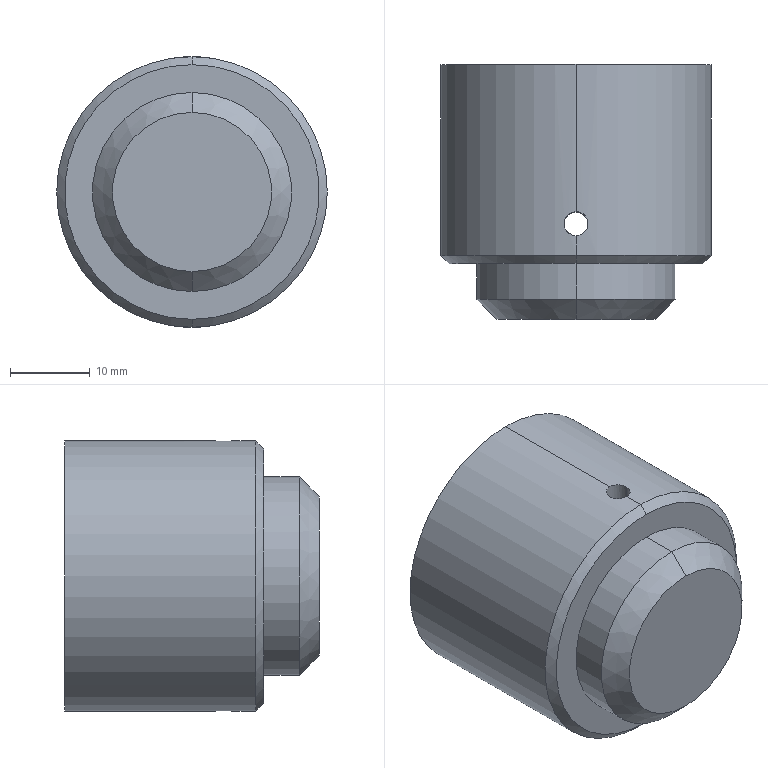Part | SolidWorks | features HoleWzd 1, ICE 1, Revolution 1 | 1 solid | 22 faces | box 34 x 32 x 34 mm | volume 12156 mm3 | cylinder 12 | cone 6 | plane 4 | commonest cylinder face diameters 3 x4 5 x2 25 x2 28 x2 34 x2
STEP:
#1=CARTESIAN_POINT('',(0.,10.5,14.));
#2=VERTEX_POINT('',#1);
#3=CARTESIAN_POINT('',(-1.5,12.,13.919));
#4=VERTEX_POINT('',#3);
#5=CARTESIAN_POINT('',(0.,10.5,14.));
#6=CARTESIAN_POINT('',(-0.09921,10.5,14.));
#7=CARTESIAN_POINT('',(-0.1967,10.51,13.999));
#8=CARTESIAN_POINT('',(-0.3886,10.548,13.995));
#9=CARTESIAN_POINT('',(-0.4839,10.577,13.992));
#10=CARTESIAN_POINT('',(-0.6656,10.652,13.984));
#11=CARTESIAN_POINT('',(-0.7518,10.698,13.98));
#12=CARTESIAN_POINT('',(-0.9148,10.807,13.97));
#13=CARTESIAN_POINT('',(-0.9919,10.871,13.965));
#14=CARTESIAN_POINT('',(-1.199,11.078,13.949));
#15=CARTESIAN_POINT('',(-1.311,11.245,13.939));
#16=CARTESIAN_POINT('',(-1.461,11.607,13.924));
#17=CARTESIAN_POINT('',(-1.5,11.804,13.919));
#18=CARTESIAN_POINT('',(-1.5,12.,13.919));
#19=B_SPLINE_CURVE_WITH_KNOTS('',3,(#5,#6,#7,#8,#9,#10,#11,#12,#13,#14,#15,#16,#17,#18),.UNSPECIFIED.,.F.,.F.,(4,2,2,2,2,2,4),(0.,0.0002934,0.0005868,0.0008802,0.001174,0.00176,0.002347),.UNSPECIFIED.);
#20=EDGE_CURVE('',#2,#4,#19,.T.);
#21=ORIENTED_EDGE('',*,*,#20,.T.);
#22=CARTESIAN_POINT('',(-1.5,12.,16.934));
#23=VERTEX_POINT('',#22);
#24=CARTESIAN_POINT('',(-1.5,12.,-35.));
#25=DIRECTION('',(0.,0.,1.));
#26=VECTOR('',#25,1000.);
#27=LINE('',#24,#26);
#28=EDGE_CURVE('',#4,#23,#27,.T.);
#29=ORIENTED_EDGE('',*,*,#28,.T.);
#30=CARTESIAN_POINT('',(0.,10.5,17.));
#31=VERTEX_POINT('',#30);
#32=CARTESIAN_POINT('',(-1.5,12.,16.934));
#33=CARTESIAN_POINT('',(-1.5,11.802,16.934));
#34=CARTESIAN_POINT('',(-1.461,11.607,16.937));
#35=CARTESIAN_POINT('',(-1.348,11.335,16.947));
#36=CARTESIAN_POINT('',(-1.302,11.249,16.95));
#37=CARTESIAN_POINT('',(-1.193,11.086,16.958));
#38=CARTESIAN_POINT('',(-1.13,11.009,16.963));
#39=CARTESIAN_POINT('',(-0.9228,10.801,16.976));
#40=CARTESIAN_POINT('',(-0.7557,10.69,16.984));
#41=CARTESIAN_POINT('',(-0.3951,10.54,16.996));
#42=CARTESIAN_POINT('',(-0.1982,10.5,17.));
#43=CARTESIAN_POINT('',(0.,10.5,17.));
#44=B_SPLINE_CURVE_WITH_KNOTS('',3,(#32,#33,#34,#35,#36,#37,#38,#39,#40,#41,#42,#43),.UNSPECIFIED.,.F.,.F.,(4,2,2,2,2,4),(0.007039,0.007625,0.007918,0.008211,0.008797,0.009383),.UNSPECIFIED.);
#45=EDGE_CURVE('',#23,#31,#44,.T.);
#46=ORIENTED_EDGE('',*,*,#45,.T.);
#47=CARTESIAN_POINT('',(1.5,12.,16.934));
#48=VERTEX_POINT('',#47);
#49=CARTESIAN_POINT('',(0.,10.5,17.));
#50=CARTESIAN_POINT('',(0.09918,10.5,17.));
#51=CARTESIAN_POINT('',(0.1967,10.51,16.999));
#52=CARTESIAN_POINT('',(0.3885,10.548,16.996));
#53=CARTESIAN_POINT('',(0.4839,10.577,16.993));
#54=CARTESIAN_POINT('',(0.6655,10.652,16.987));
#55=CARTESIAN_POINT('',(0.7517,10.698,16.984));
#56=CARTESIAN_POINT('',(0.9147,10.807,16.976));
#57=CARTESIAN_POINT('',(0.9919,10.871,16.971));
#58=CARTESIAN_POINT('',(1.199,11.078,16.958));
#59=CARTESIAN_POINT('',(1.311,11.246,16.95));
#60=CARTESIAN_POINT('',(1.461,11.607,16.937));
#61=CARTESIAN_POINT('',(1.5,11.804,16.934));
#62=CARTESIAN_POINT('',(1.5,12.,16.934));
#63=B_SPLINE_CURVE_WITH_KNOTS('',3,(#49,#50,#51,#52,#53,#54,#55,#56,#57,#58,#59,#60,#61,#62),.UNSPECIFIED.,.F.,.F.,(4,2,2,2,2,2,4),(0.,0.0002933,0.0005866,0.0008799,0.001173,0.00176,0.002347),.UNSPECIFIED.);
#64=EDGE_CURVE('',#31,#48,#63,.T.);
#65=ORIENTED_EDGE('',*,*,#64,.T.);
#66=CARTESIAN_POINT('',(1.5,12.,13.919));
#67=VERTEX_POINT('',#66);
#68=CARTESIAN_POINT('',(1.5,12.,-35.));
#69=DIRECTION('',(0.,0.,1.));
#70=VECTOR('',#69,1000.);
#71=LINE('',#68,#70);
#72=EDGE_CURVE('',#67,#48,#71,.T.);
#73=ORIENTED_EDGE('',*,*,#72,.F.);
#74=CARTESIAN_POINT('',(1.5,12.,13.919));
#75=CARTESIAN_POINT('',(1.5,11.901,13.919));
#76=CARTESIAN_POINT('',(1.49,11.803,13.92));
#77=CARTESIAN_POINT('',(1.452,11.612,13.924));
#78=CARTESIAN_POINT('',(1.423,11.516,13.928));
#79=CARTESIAN_POINT('',(1.348,11.335,13.935));
#80=CARTESIAN_POINT('',(1.302,11.249,13.939));
#81=CARTESIAN_POINT('',(1.193,11.086,13.949));
#82=CARTESIAN_POINT('',(1.13,11.009,13.954));
#83=CARTESIAN_POINT('',(0.9228,10.801,13.97));
#84=CARTESIAN_POINT('',(0.7558,10.69,13.981));
#85=CARTESIAN_POINT('',(0.3952,10.54,13.996));
#86=CARTESIAN_POINT('',(0.1982,10.5,14.));
#87=CARTESIAN_POINT('',(0.,10.5,14.));
#88=B_SPLINE_CURVE_WITH_KNOTS('',3,(#74,#75,#76,#77,#78,#79,#80,#81,#82,#83,#84,#85,#86,#87),.UNSPECIFIED.,.F.,.F.,(4,2,2,2,2,2,4),(0.00704,0.007333,0.007626,0.007919,0.008213,0.008799,0.009385),.UNSPECIFIED.);
#89=EDGE_CURVE('',#67,#2,#88,.T.);
#90=ORIENTED_EDGE('',*,*,#89,.T.);
#91=EDGE_LOOP('',(#21,#29,#46,#65,#73,#90));
#92=FACE_OUTER_BOUND('',#91,.T.);
#93=CARTESIAN_POINT('',(0.,12.,-35.));
#94=DIRECTION('',(0.,0.,1.));
#95=DIRECTION('',(1.,0.,0.));
#96=AXIS2_PLACEMENT_3D('',#93,#94,#95);
#97=CYLINDRICAL_SURFACE('',#96,1.5);
#98=ADVANCED_FACE('',(#92),#97,.F.);
#99=CARTESIAN_POINT('',(0.,10.5,-17.));
#100=VERTEX_POINT('',#99);
#101=CARTESIAN_POINT('',(-1.5,12.,-16.934));
#102=VERTEX_POINT('',#101);
#103=CARTESIAN_POINT('',(0.,10.5,-17.));
#104=CARTESIAN_POINT('',(-0.09787,10.5,-17.));
#105=CARTESIAN_POINT('',(-0.1973,10.51,-16.999));
#106=CARTESIAN_POINT('',(-0.3896,10.548,-16.996));
#107=CARTESIAN_POINT('',(-0.4831,10.577,-16.993));
#108=CARTESIAN_POINT('',(-0.6648,10.652,-16.987));
#109=CARTESIAN_POINT('',(-0.7525,10.699,-16.984));
#110=CARTESIAN_POINT('',(-0.9149,10.807,-16.976));
#111=CARTESIAN_POINT('',(-0.9907,10.869,-16.971));
#112=CARTESIAN_POINT('',(-1.131,11.009,-16.963));
#113=CARTESIAN_POINT('',(-1.193,11.085,-16.958));
#114=CARTESIAN_POINT('',(-1.301,11.248,-16.95));
#115=CARTESIAN_POINT('',(-1.348,11.335,-16.946));
#116=CARTESIAN_POINT('',(-1.423,11.517,-16.94));
#117=CARTESIAN_POINT('',(-1.452,11.61,-16.938));
#118=CARTESIAN_POINT('',(-1.49,11.803,-16.935));
#119=CARTESIAN_POINT('',(-1.5,11.902,-16.934));
#120=CARTESIAN_POINT('',(-1.5,12.,-16.934));
#121=B_SPLINE_CURVE_WITH_KNOTS('',3,(#103,#104,#105,#106,#107,#108,#109,#110,#111,#112,#113,#114,#115,#116,#117,#118,#119,#120),.UNSPECIFIED.,.F.,.F.,(4,2,2,2,2,2,2,2,4),(0.002347,0.00264,0.002933,0.003226,0.003519,0.003812,0.004106,0.004399,0.004692),.UNSPECIFIED.);
#122=EDGE_CURVE('',#100,#102,#121,.T.);
#123=ORIENTED_EDGE('',*,*,#122,.T.);
#124=CARTESIAN_POINT('',(-1.5,12.,-13.919));
#125=VERTEX_POINT('',#124);
#126=CARTESIAN_POINT('',(-1.5,12.,-35.));
#127=DIRECTION('',(0.,0.,1.));
#128=VECTOR('',#127,1000.);
#129=LINE('',#126,#128);
#130=EDGE_CURVE('',#102,#125,#129,.T.);
#131=ORIENTED_EDGE('',*,*,#130,.T.);
#132=CARTESIAN_POINT('',(0.,10.5,-14.));
#133=VERTEX_POINT('',#132);
#134=CARTESIAN_POINT('',(-1.5,12.,-13.919));
#135=CARTESIAN_POINT('',(-1.5,11.804,-13.919));
#136=CARTESIAN_POINT('',(-1.461,11.607,-13.924));
#137=CARTESIAN_POINT('',(-1.311,11.245,-13.939));
#138=CARTESIAN_POINT('',(-1.199,11.078,-13.949));
#139=CARTESIAN_POINT('',(-0.9918,10.87,-13.965));
#140=CARTESIAN_POINT('',(-0.9147,10.807,-13.97));
#141=CARTESIAN_POINT('',(-0.7517,10.698,-13.98));
#142=CARTESIAN_POINT('',(-0.6656,10.652,-13.984));
#143=CARTESIAN_POINT('',(-0.4839,10.577,-13.992));
#144=CARTESIAN_POINT('',(-0.3886,10.548,-13.995));
#145=CARTESIAN_POINT('',(-0.1967,10.51,-13.999));
#146=CARTESIAN_POINT('',(-0.09918,10.5,-14.));
#147=CARTESIAN_POINT('',(0.,10.5,-14.));
#148=B_SPLINE_CURVE_WITH_KNOTS('',3,(#134,#135,#136,#137,#138,#139,#140,#141,#142,#143,#144,#145,#146,#147),.UNSPECIFIED.,.F.,.F.,(4,2,2,2,2,2,4),(0.004693,0.00528,0.005867,0.00616,0.006453,0.006747,0.00704),.UNSPECIFIED.);
#149=EDGE_CURVE('',#125,#133,#148,.T.);
#150=ORIENTED_EDGE('',*,*,#149,.T.);
#151=CARTESIAN_POINT('',(1.5,12.,-13.919));
#152=VERTEX_POINT('',#151);
#153=CARTESIAN_POINT('',(0.,10.5,-14.));
#154=CARTESIAN_POINT('',(0.09909,10.5,-14.));
#155=CARTESIAN_POINT('',(0.1966,10.51,-13.999));
#156=CARTESIAN_POINT('',(0.3883,10.548,-13.995));
#157=CARTESIAN_POINT('',(0.4835,10.577,-13.992));
#158=CARTESIAN_POINT('',(0.6651,10.652,-13.984));
#159=CARTESIAN_POINT('',(0.7512,10.698,-13.98));
#160=CARTESIAN_POINT('',(0.9141,10.807,-13.97));
#161=CARTESIAN_POINT('',(0.9912,10.87,-13.965));
#162=CARTESIAN_POINT('',(1.199,11.077,-13.949));
#163=CARTESIAN_POINT('',(1.31,11.244,-13.939));
#164=CARTESIAN_POINT('',(1.46,11.605,-13.924));
#165=CARTESIAN_POINT('',(1.5,11.802,-13.919));
#166=CARTESIAN_POINT('',(1.5,12.,-13.919));
#167=B_SPLINE_CURVE_WITH_KNOTS('',3,(#153,#154,#155,#156,#157,#158,#159,#160,#161,#162,#163,#164,#165,#166),.UNSPECIFIED.,.F.,.F.,(4,2,2,2,2,2,4),(0.00704,0.007333,0.007626,0.007919,0.008213,0.008799,0.009385),.UNSPECIFIED.);
#168=EDGE_CURVE('',#133,#152,#167,.T.);
#169=ORIENTED_EDGE('',*,*,#168,.T.);
#170=CARTESIAN_POINT('',(1.5,12.,-16.934));
#171=VERTEX_POINT('',#170);
#172=CARTESIAN_POINT('',(1.5,12.,-35.));
#173=DIRECTION('',(0.,0.,1.));
#174=VECTOR('',#173,1000.);
#175=LINE('',#172,#174);
#176=EDGE_CURVE('',#171,#152,#175,.T.);
#177=ORIENTED_EDGE('',*,*,#176,.F.);
#178=CARTESIAN_POINT('',(1.5,12.,-16.934));
#179=CARTESIAN_POINT('',(1.5,11.901,-16.934));
#180=CARTESIAN_POINT('',(1.49,11.803,-16.935));
#181=CARTESIAN_POINT('',(1.452,11.611,-16.938));
#182=CARTESIAN_POINT('',(1.423,11.516,-16.94));
#183=CARTESIAN_POINT('',(1.348,11.334,-16.947));
#184=CARTESIAN_POINT('',(1.302,11.248,-16.95));
#185=CARTESIAN_POINT('',(1.193,11.085,-16.958));
#186=CARTESIAN_POINT('',(1.129,11.008,-16.963));
#187=CARTESIAN_POINT('',(0.9219,10.801,-16.976));
#188=CARTESIAN_POINT('',(0.7545,10.689,-16.984));
#189=CARTESIAN_POINT('',(0.3934,10.539,-16.996));
#190=CARTESIAN_POINT('',(0.1958,10.5,-17.));
#191=CARTESIAN_POINT('',(0.,10.5,-17.));
#192=B_SPLINE_CURVE_WITH_KNOTS('',3,(#178,#179,#180,#181,#182,#183,#184,#185,#186,#187,#188,#189,#190,#191),.UNSPECIFIED.,.F.,.F.,(4,2,2,2,2,2,4),(0.,0.0002933,0.0005866,0.0008799,0.001173,0.00176,0.002347),.UNSPECIFIED.);
#193=EDGE_CURVE('',#171,#100,#192,.T.);
#194=ORIENTED_EDGE('',*,*,#193,.T.);
#195=EDGE_LOOP('',(#123,#131,#150,#169,#177,#194));
#196=FACE_OUTER_BOUND('',#195,.T.);
#197=CARTESIAN_POINT('',(0.,12.,-35.));
#198=DIRECTION('',(0.,0.,1.));
#199=DIRECTION('',(1.,0.,0.));
#200=AXIS2_PLACEMENT_3D('',#197,#198,#199);
#201=CYLINDRICAL_SURFACE('',#200,1.5);
#202=ADVANCED_FACE('',(#196),#201,.F.);
#203=CARTESIAN_POINT('',(0.,5.,-2.5));
#204=VERTEX_POINT('',#203);
#205=CARTESIAN_POINT('',(0.,5.,2.5));
#206=VERTEX_POINT('',#205);
#207=CARTESIAN_POINT('',(0.,5.,0.));
#208=DIRECTION('',(0.,1.,0.));
#209=DIRECTION('',(0.,0.,1.));
#210=AXIS2_PLACEMENT_3D('',#207,#208,#209);
#211=CIRCLE('',#210,2.5);
#212=EDGE_CURVE('',#204,#206,#211,.T.);
#213=ORIENTED_EDGE('',*,*,#212,.F.);
#214=CARTESIAN_POINT('',(0.,10.,-2.5));
#215=VERTEX_POINT('',#214);
#216=CARTESIAN_POINT('',(0.,10.,-2.5));
#217=DIRECTION('',(0.,1.,0.));
#218=VECTOR('',#217,1000.);
#219=LINE('',#216,#218);
#220=EDGE_CURVE('',#204,#215,#219,.T.);
#221=ORIENTED_EDGE('',*,*,#220,.T.);
#222=CARTESIAN_POINT('',(0.,10.,2.5));
#223=VERTEX_POINT('',#222);
#224=CARTESIAN_POINT('',(0.,10.,0.));
#225=DIRECTION('',(0.,1.,0.));
#226=DIRECTION('',(0.,0.,1.));
#227=AXIS2_PLACEMENT_3D('',#224,#225,#226);
#228=CIRCLE('',#227,2.5);
#229=EDGE_CURVE('',#215,#223,#228,.T.);
#230=ORIENTED_EDGE('',*,*,#229,.T.);
#231=CARTESIAN_POINT('',(0.,10.,2.5));
#232=DIRECTION('',(0.,1.,0.));
#233=VECTOR('',#232,1000.);
#234=LINE('',#231,#233);
#235=EDGE_CURVE('',#206,#223,#234,.T.);
#236=ORIENTED_EDGE('',*,*,#235,.F.);
#237=EDGE_LOOP('',(#213,#221,#230,#236));
#238=FACE_OUTER_BOUND('',#237,.T.);
#239=CARTESIAN_POINT('',(0.,10.,0.));
#240=DIRECTION('',(0.,1.,0.));
#241=DIRECTION('',(0.,0.,1.));
#242=AXIS2_PLACEMENT_3D('',#239,#240,#241);
#243=CYLINDRICAL_SURFACE('',#242,2.5);
#244=ADVANCED_FACE('',(#238),#243,.F.);
#245=CARTESIAN_POINT('',(0.,3.498,0.));
#246=VERTEX_POINT('',#245);
#247=CARTESIAN_POINT('',(0.,5.,2.5));
#248=DIRECTION('',(0.,0.515,0.8572));
#249=VECTOR('',#248,1000.);
#250=LINE('',#247,#249);
#251=EDGE_CURVE('',#246,#206,#250,.T.);
#252=ORIENTED_EDGE('',*,*,#251,.F.);
#253=CARTESIAN_POINT('',(0.,5.,-2.5));
#254=DIRECTION('',(0.,0.515,-0.8572));
#255=VECTOR('',#254,1000.);
#256=LINE('',#253,#255);
#257=EDGE_CURVE('',#246,#204,#256,.T.);
#258=ORIENTED_EDGE('',*,*,#257,.T.);
#259=ORIENTED_EDGE('',*,*,#212,.T.);
#260=EDGE_LOOP('',(#252,#258,#259));
#261=FACE_OUTER_BOUND('',#260,.T.);
#262=CARTESIAN_POINT('',(0.,5.,0.));
#263=DIRECTION('',(0.,1.,0.));
#264=DIRECTION('',(0.,0.,1.));
#265=AXIS2_PLACEMENT_3D('',#262,#263,#264);
#266=CONICAL_SURFACE('',#265,2.5,1.03);
#267=ADVANCED_FACE('',(#261),#266,.F.);
#268=CARTESIAN_POINT('',(0.,10.,-14.));
#269=VERTEX_POINT('',#268);
#270=CARTESIAN_POINT('',(0.,10.,14.));
#271=VERTEX_POINT('',#270);
#272=CARTESIAN_POINT('',(0.,10.,0.));
#273=DIRECTION('',(0.,1.,0.));
#274=DIRECTION('',(0.,0.,1.));
#275=AXIS2_PLACEMENT_3D('',#272,#273,#274);
#276=CIRCLE('',#275,14.);
#277=EDGE_CURVE('',#269,#271,#276,.T.);
#278=ORIENTED_EDGE('',*,*,#277,.F.);
#279=CARTESIAN_POINT('',(0.,19.381,-14.));
#280=DIRECTION('',(0.,1.,0.));
#281=VECTOR('',#280,1000.);
#282=LINE('',#279,#281);
#283=EDGE_CURVE('',#269,#133,#282,.T.);
#284=ORIENTED_EDGE('',*,*,#283,.T.);
#285=ORIENTED_EDGE('',*,*,#149,.F.);
#286=CARTESIAN_POINT('',(0.,13.5,-14.));
#287=VERTEX_POINT('',#286);
#288=CARTESIAN_POINT('',(0.,13.5,-14.));
#289=CARTESIAN_POINT('',(-0.09789,13.5,-14.));
#290=CARTESIAN_POINT('',(-0.1973,13.49,-13.999));
#291=CARTESIAN_POINT('',(-0.3897,13.452,-13.995));
#292=CARTESIAN_POINT('',(-0.4832,13.423,-13.992));
#293=CARTESIAN_POINT('',(-0.6649,13.348,-13.984));
#294=CARTESIAN_POINT('',(-0.7526,13.301,-13.98));
#295=CARTESIAN_POINT('',(-0.915,13.193,-13.97));
#296=CARTESIAN_POINT('',(-0.9907,13.131,-13.965));
#297=CARTESIAN_POINT('',(-1.131,12.991,-13.954));
#298=CARTESIAN_POINT('',(-1.193,12.915,-13.949));
#299=CARTESIAN_POINT('',(-1.301,12.753,-13.94));
#300=CARTESIAN_POINT('',(-1.348,12.665,-13.935));
#301=CARTESIAN_POINT('',(-1.423,12.483,-13.927));
#302=CARTESIAN_POINT('',(-1.452,12.39,-13.925));
#303=CARTESIAN_POINT('',(-1.49,12.197,-13.92));
#304=CARTESIAN_POINT('',(-1.5,12.098,-13.919));
#305=CARTESIAN_POINT('',(-1.5,12.,-13.919));
#306=B_SPLINE_CURVE_WITH_KNOTS('',3,(#288,#289,#290,#291,#292,#293,#294,#295,#296,#297,#298,#299,#300,#301,#302,#303,#304,#305),.UNSPECIFIED.,.F.,.F.,(4,2,2,2,2,2,2,2,4),(0.002347,0.00264,0.002934,0.003227,0.00352,0.003813,0.004107,0.0044,0.004693),.UNSPECIFIED.);
#307=EDGE_CURVE('',#287,#125,#306,.T.);
#308=ORIENTED_EDGE('',*,*,#307,.F.);
#309=CARTESIAN_POINT('',(0.,32.,-14.));
#310=VERTEX_POINT('',#309);
#311=CARTESIAN_POINT('',(0.,19.381,-14.));
#312=DIRECTION('',(0.,1.,0.));
#313=VECTOR('',#312,1000.);
#314=LINE('',#311,#313);
#315=EDGE_CURVE('',#287,#310,#314,.T.);
#316=ORIENTED_EDGE('',*,*,#315,.T.);
#317=CARTESIAN_POINT('',(0.,32.,14.));
#318=VERTEX_POINT('',#317);
#319=CARTESIAN_POINT('',(0.,32.,0.));
#320=DIRECTION('',(0.,1.,0.));
#321=DIRECTION('',(0.,0.,1.));
#322=AXIS2_PLACEMENT_3D('',#319,#320,#321);
#323=CIRCLE('',#322,14.);
#324=EDGE_CURVE('',#310,#318,#323,.T.);
#325=ORIENTED_EDGE('',*,*,#324,.T.);
#326=CARTESIAN_POINT('',(0.,13.5,14.));
#327=VERTEX_POINT('',#326);
#328=CARTESIAN_POINT('',(0.,19.381,14.));
#329=DIRECTION('',(0.,1.,0.));
#330=VECTOR('',#329,1000.);
#331=LINE('',#328,#330);
#332=EDGE_CURVE('',#327,#318,#331,.T.);
#333=ORIENTED_EDGE('',*,*,#332,.F.);
#334=CARTESIAN_POINT('',(-1.5,12.,13.919));
#335=CARTESIAN_POINT('',(-1.5,12.098,13.919));
#336=CARTESIAN_POINT('',(-1.49,12.197,13.92));
#337=CARTESIAN_POINT('',(-1.452,12.39,13.925));
#338=CARTESIAN_POINT('',(-1.423,12.483,13.928));
#339=CARTESIAN_POINT('',(-1.348,12.665,13.935));
#340=CARTESIAN_POINT('',(-1.301,12.753,13.94));
#341=CARTESIAN_POINT('',(-1.193,12.915,13.949));
#342=CARTESIAN_POINT('',(-1.131,12.991,13.954));
#343=CARTESIAN_POINT('',(-0.9906,13.131,13.965));
#344=CARTESIAN_POINT('',(-0.9149,13.193,13.97));
#345=CARTESIAN_POINT('',(-0.7525,13.301,13.98));
#346=CARTESIAN_POINT('',(-0.6648,13.348,13.985));
#347=CARTESIAN_POINT('',(-0.4832,13.423,13.992));
#348=CARTESIAN_POINT('',(-0.3897,13.452,13.995));
#349=CARTESIAN_POINT('',(-0.1974,13.49,13.999));
#350=CARTESIAN_POINT('',(-0.09791,13.5,14.));
#351=CARTESIAN_POINT('',(0.,13.5,14.));
#352=B_SPLINE_CURVE_WITH_KNOTS('',3,(#334,#335,#336,#337,#338,#339,#340,#341,#342,#343,#344,#345,#346,#347,#348,#349,#350,#351),.UNSPECIFIED.,.F.,.F.,(4,2,2,2,2,2,2,2,4),(0.002347,0.00264,0.002934,0.003227,0.00352,0.003813,0.004107,0.0044,0.004693),.UNSPECIFIED.);
#353=EDGE_CURVE('',#4,#327,#352,.T.);
#354=ORIENTED_EDGE('',*,*,#353,.F.);
#355=ORIENTED_EDGE('',*,*,#20,.F.);
#356=CARTESIAN_POINT('',(0.,19.381,14.));
#357=DIRECTION('',(0.,1.,0.));
#358=VECTOR('',#357,1000.);
#359=LINE('',#356,#358);
#360=EDGE_CURVE('',#271,#2,#359,.T.);
#361=ORIENTED_EDGE('',*,*,#360,.F.);
#362=EDGE_LOOP('',(#278,#284,#285,#308,#316,#325,#333,#354,#355,#361));
#363=FACE_OUTER_BOUND('',#362,.T.);
#364=CARTESIAN_POINT('',(0.,19.381,0.));
#365=DIRECTION('',(0.,1.,0.));
#366=DIRECTION('',(0.,0.,1.));
#367=AXIS2_PLACEMENT_3D('',#364,#365,#366);
#368=CYLINDRICAL_SURFACE('',#367,14.);
#369=ADVANCED_FACE('',(#363),#368,.F.);
#370=CARTESIAN_POINT('',(0.,8.,17.));
#371=VERTEX_POINT('',#370);
#372=CARTESIAN_POINT('',(0.,8.,-17.));
#373=VERTEX_POINT('',#372);
#374=CARTESIAN_POINT('',(0.,8.,0.));
#375=DIRECTION('',(0.,1.,0.));
#376=DIRECTION('',(0.,0.,1.));
#377=AXIS2_PLACEMENT_3D('',#374,#375,#376);
#378=CIRCLE('',#377,17.);
#379=EDGE_CURVE('',#371,#373,#378,.T.);
#380=ORIENTED_EDGE('',*,*,#379,.T.);
#381=CARTESIAN_POINT('',(0.,19.381,-17.));
#382=DIRECTION('',(0.,1.,0.));
#383=VECTOR('',#382,1000.);
#384=LINE('',#381,#383);
#385=EDGE_CURVE('',#373,#100,#384,.T.);
#386=ORIENTED_EDGE('',*,*,#385,.T.);
#387=ORIENTED_EDGE('',*,*,#193,.F.);
#388=CARTESIAN_POINT('',(0.,13.5,-17.));
#389=VERTEX_POINT('',#388);
#390=CARTESIAN_POINT('',(0.,13.5,-17.));
#391=CARTESIAN_POINT('',(0.198,13.5,-17.));
#392=CARTESIAN_POINT('',(0.3926,13.461,-16.996));
#393=CARTESIAN_POINT('',(0.665,13.348,-16.987));
#394=CARTESIAN_POINT('',(0.7511,13.302,-16.984));
#395=CARTESIAN_POINT('',(0.914,13.193,-16.976));
#396=CARTESIAN_POINT('',(0.9912,13.13,-16.971));
#397=CARTESIAN_POINT('',(1.199,12.923,-16.958));
#398=CARTESIAN_POINT('',(1.31,12.756,-16.95));
#399=CARTESIAN_POINT('',(1.46,12.395,-16.937));
#400=CARTESIAN_POINT('',(1.5,12.198,-16.934));
#401=CARTESIAN_POINT('',(1.5,12.,-16.934));
#402=B_SPLINE_CURVE_WITH_KNOTS('',3,(#390,#391,#392,#393,#394,#395,#396,#397,#398,#399,#400,#401),.UNSPECIFIED.,.F.,.F.,(4,2,2,2,2,4),(0.007039,0.007625,0.007918,0.008211,0.008797,0.009383),.UNSPECIFIED.);
#403=EDGE_CURVE('',#389,#171,#402,.T.);
#404=ORIENTED_EDGE('',*,*,#403,.F.);
#405=CARTESIAN_POINT('',(0.,32.,-17.));
#406=VERTEX_POINT('',#405);
#407=CARTESIAN_POINT('',(0.,19.381,-17.));
#408=DIRECTION('',(0.,1.,0.));
#409=VECTOR('',#408,1000.);
#410=LINE('',#407,#409);
#411=EDGE_CURVE('',#389,#406,#410,.T.);
#412=ORIENTED_EDGE('',*,*,#411,.T.);
#413=CARTESIAN_POINT('',(0.,32.,17.));
#414=VERTEX_POINT('',#413);
#415=CARTESIAN_POINT('',(0.,32.,0.));
#416=DIRECTION('',(0.,1.,0.));
#417=DIRECTION('',(0.,0.,1.));
#418=AXIS2_PLACEMENT_3D('',#415,#416,#417);
#419=CIRCLE('',#418,17.);
#420=EDGE_CURVE('',#414,#406,#419,.T.);
#421=ORIENTED_EDGE('',*,*,#420,.F.);
#422=CARTESIAN_POINT('',(0.,13.5,17.));
#423=VERTEX_POINT('',#422);
#424=CARTESIAN_POINT('',(0.,19.381,17.));
#425=DIRECTION('',(0.,1.,0.));
#426=VECTOR('',#425,1000.);
#427=LINE('',#424,#426);
#428=EDGE_CURVE('',#423,#414,#427,.T.);
#429=ORIENTED_EDGE('',*,*,#428,.F.);
#430=CARTESIAN_POINT('',(1.5,12.,16.934));
#431=CARTESIAN_POINT('',(1.5,12.098,16.934));
#432=CARTESIAN_POINT('',(1.49,12.197,16.935));
#433=CARTESIAN_POINT('',(1.452,12.39,16.938));
#434=CARTESIAN_POINT('',(1.423,12.483,16.94));
#435=CARTESIAN_POINT('',(1.348,12.665,16.946));
#436=CARTESIAN_POINT('',(1.301,12.752,16.95));
#437=CARTESIAN_POINT('',(1.193,12.915,16.958));
#438=CARTESIAN_POINT('',(1.131,12.991,16.963));
#439=CARTESIAN_POINT('',(0.9906,13.131,16.971));
#440=CARTESIAN_POINT('',(0.9149,13.193,16.976));
#441=CARTESIAN_POINT('',(0.7525,13.301,16.984));
#442=CARTESIAN_POINT('',(0.6648,13.348,16.987));
#443=CARTESIAN_POINT('',(0.4831,13.423,16.993));
#444=CARTESIAN_POINT('',(0.3896,13.452,16.996));
#445=CARTESIAN_POINT('',(0.1973,13.49,16.999));
#446=CARTESIAN_POINT('',(0.0979,13.5,17.));
#447=CARTESIAN_POINT('',(0.,13.5,17.));
#448=B_SPLINE_CURVE_WITH_KNOTS('',3,(#430,#431,#432,#433,#434,#435,#436,#437,#438,#439,#440,#441,#442,#443,#444,#445,#446,#447),.UNSPECIFIED.,.F.,.F.,(4,2,2,2,2,2,2,2,4),(0.002347,0.00264,0.002933,0.003226,0.003519,0.003812,0.004106,0.004399,0.004692),.UNSPECIFIED.);
#449=EDGE_CURVE('',#48,#423,#448,.T.);
#450=ORIENTED_EDGE('',*,*,#449,.F.);
#451=ORIENTED_EDGE('',*,*,#64,.F.);
#452=CARTESIAN_POINT('',(0.,19.381,17.));
#453=DIRECTION('',(0.,1.,0.));
#454=VECTOR('',#453,1000.);
#455=LINE('',#452,#454);
#456=EDGE_CURVE('',#371,#31,#455,.T.);
#457=ORIENTED_EDGE('',*,*,#456,.F.);
#458=EDGE_LOOP('',(#380,#386,#387,#404,#412,#421,#429,#450,#451,#457));
#459=FACE_OUTER_BOUND('',#458,.T.);
#460=CARTESIAN_POINT('',(0.,19.381,0.));
#461=DIRECTION('',(0.,1.,0.));
#462=DIRECTION('',(0.,0.,1.));
#463=AXIS2_PLACEMENT_3D('',#460,#461,#462);
#464=CYLINDRICAL_SURFACE('',#463,17.);
#465=ADVANCED_FACE('',(#459),#464,.T.);
#466=CARTESIAN_POINT('',(0.,7.,16.));
#467=VERTEX_POINT('',#466);
#468=CARTESIAN_POINT('',(0.,7.,-16.));
#469=VERTEX_POINT('',#468);
#470=CARTESIAN_POINT('',(0.,7.,0.));
#471=DIRECTION('',(0.,1.,0.));
#472=DIRECTION('',(0.,0.,1.));
#473=AXIS2_PLACEMENT_3D('',#470,#471,#472);
#474=CIRCLE('',#473,16.);
#475=EDGE_CURVE('',#467,#469,#474,.T.);
#476=ORIENTED_EDGE('',*,*,#475,.T.);
#477=CARTESIAN_POINT('',(0.,8.,-17.));
#478=DIRECTION('',(0.,0.7071,-0.7071));
#479=VECTOR('',#478,1000.);
#480=LINE('',#477,#479);
#481=EDGE_CURVE('',#469,#373,#480,.T.);
#482=ORIENTED_EDGE('',*,*,#481,.T.);
#483=ORIENTED_EDGE('',*,*,#379,.F.);
#484=CARTESIAN_POINT('',(0.,8.,17.));
#485=DIRECTION('',(0.,0.7071,0.7071));
#486=VECTOR('',#485,1000.);
#487=LINE('',#484,#486);
#488=EDGE_CURVE('',#467,#371,#487,.T.);
#489=ORIENTED_EDGE('',*,*,#488,.F.);
#490=EDGE_LOOP('',(#476,#482,#483,#489));
#491=FACE_OUTER_BOUND('',#490,.T.);
#492=CARTESIAN_POINT('',(0.,8.,0.));
#493=DIRECTION('',(0.,1.,0.));
#494=DIRECTION('',(0.,0.,1.));
#495=AXIS2_PLACEMENT_3D('',#492,#493,#494);
#496=CONICAL_SURFACE('',#495,17.,0.7854);
#497=ADVANCED_FACE('',(#491),#496,.T.);
#498=CARTESIAN_POINT('',(0.,2.5,12.5));
#499=VERTEX_POINT('',#498);
#500=CARTESIAN_POINT('',(0.,2.5,-12.5));
#501=VERTEX_POINT('',#500);
#502=CARTESIAN_POINT('',(0.,2.5,0.));
#503=DIRECTION('',(0.,1.,0.));
#504=DIRECTION('',(0.,0.,1.));
#505=AXIS2_PLACEMENT_3D('',#502,#503,#504);
#506=CIRCLE('',#505,12.5);
#507=EDGE_CURVE('',#499,#501,#506,.T.);
#508=ORIENTED_EDGE('',*,*,#507,.T.);
#509=CARTESIAN_POINT('',(0.,7.,-12.5));
#510=VERTEX_POINT('',#509);
#511=CARTESIAN_POINT('',(0.,19.381,-12.5));
#512=DIRECTION('',(0.,1.,0.));
#513=VECTOR('',#512,1000.);
#514=LINE('',#511,#513);
#515=EDGE_CURVE('',#501,#510,#514,.T.);
#516=ORIENTED_EDGE('',*,*,#515,.T.);
#517=CARTESIAN_POINT('',(0.,7.,12.5));
#518=VERTEX_POINT('',#517);
#519=CARTESIAN_POINT('',(0.,7.,0.));
#520=DIRECTION('',(0.,1.,0.));
#521=DIRECTION('',(0.,0.,1.));
#522=AXIS2_PLACEMENT_3D('',#519,#520,#521);
#523=CIRCLE('',#522,12.5);
#524=EDGE_CURVE('',#518,#510,#523,.T.);
#525=ORIENTED_EDGE('',*,*,#524,.F.);
#526=CARTESIAN_POINT('',(0.,19.381,12.5));
#527=DIRECTION('',(0.,1.,0.));
#528=VECTOR('',#527,1000.);
#529=LINE('',#526,#528);
#530=EDGE_CURVE('',#499,#518,#529,.T.);
#531=ORIENTED_EDGE('',*,*,#530,.F.);
#532=EDGE_LOOP('',(#508,#516,#525,#531));
#533=FACE_OUTER_BOUND('',#532,.T.);
#534=CARTESIAN_POINT('',(0.,19.381,0.));
#535=DIRECTION('',(0.,1.,0.));
#536=DIRECTION('',(0.,0.,1.));
#537=AXIS2_PLACEMENT_3D('',#534,#535,#536);
#538=CYLINDRICAL_SURFACE('',#537,12.5);
#539=ADVANCED_FACE('',(#533),#538,.T.);
#540=CARTESIAN_POINT('',(0.,0.,10.));
#541=VERTEX_POINT('',#540);
#542=CARTESIAN_POINT('',(0.,0.,-10.));
#543=VERTEX_POINT('',#542);
#544=CARTESIAN_POINT('',(0.,0.,0.));
#545=DIRECTION('',(0.,1.,0.));
#546=DIRECTION('',(0.,0.,1.));
#547=AXIS2_PLACEMENT_3D('',#544,#545,#546);
#548=CIRCLE('',#547,10.);
#549=EDGE_CURVE('',#541,#543,#548,.T.);
#550=ORIENTED_EDGE('',*,*,#549,.T.);
#551=CARTESIAN_POINT('',(0.,2.5,-12.5));
#552=DIRECTION('',(0.,0.7071,-0.7071));
#553=VECTOR('',#552,1000.);
#554=LINE('',#551,#553);
#555=EDGE_CURVE('',#543,#501,#554,.T.);
#556=ORIENTED_EDGE('',*,*,#555,.T.);
#557=ORIENTED_EDGE('',*,*,#507,.F.);
#558=CARTESIAN_POINT('',(0.,2.5,12.5));
#559=DIRECTION('',(0.,0.7071,0.7071));
#560=VECTOR('',#559,1000.);
#561=LINE('',#558,#560);
#562=EDGE_CURVE('',#541,#499,#561,.T.);
#563=ORIENTED_EDGE('',*,*,#562,.F.);
#564=EDGE_LOOP('',(#550,#556,#557,#563));
#565=FACE_OUTER_BOUND('',#564,.T.);
#566=CARTESIAN_POINT('',(0.,2.5,0.));
#567=DIRECTION('',(0.,1.,0.));
#568=DIRECTION('',(0.,0.,1.));
#569=AXIS2_PLACEMENT_3D('',#566,#567,#568);
#570=CONICAL_SURFACE('',#569,12.5,0.7854);
#571=ADVANCED_FACE('',(#565),#570,.T.);
#572=ORIENTED_EDGE('',*,*,#549,.F.);
#573=CARTESIAN_POINT('',(0.,0.,0.));
#574=DIRECTION('',(0.,1.,0.));
#575=DIRECTION('',(0.,0.,1.));
#576=AXIS2_PLACEMENT_3D('',#573,#574,#575);
#577=CIRCLE('',#576,10.);
#578=EDGE_CURVE('',#543,#541,#577,.T.);
#579=ORIENTED_EDGE('',*,*,#578,.F.);
#580=EDGE_LOOP('',(#572,#579));
#581=FACE_OUTER_BOUND('',#580,.T.);
#582=CARTESIAN_POINT('',(0.,0.,0.));
#583=DIRECTION('',(0.,-1.,0.));
#584=DIRECTION('',(0.,0.,-1.));
#585=AXIS2_PLACEMENT_3D('',#582,#583,#584);
#586=PLANE('',#585);
#587=ADVANCED_FACE('',(#581),#586,.T.);
#588=ORIENTED_EDGE('',*,*,#555,.F.);
#589=ORIENTED_EDGE('',*,*,#578,.T.);
#590=ORIENTED_EDGE('',*,*,#562,.T.);
#591=CARTESIAN_POINT('',(0.,2.5,0.));
#592=DIRECTION('',(0.,1.,0.));
#593=DIRECTION('',(0.,0.,1.));
#594=AXIS2_PLACEMENT_3D('',#591,#592,#593);
#595=CIRCLE('',#594,12.5);
#596=EDGE_CURVE('',#501,#499,#595,.T.);
#597=ORIENTED_EDGE('',*,*,#596,.F.);
#598=EDGE_LOOP('',(#588,#589,#590,#597));
#599=FACE_OUTER_BOUND('',#598,.T.);
#600=CARTESIAN_POINT('',(0.,2.5,0.));
#601=DIRECTION('',(0.,1.,0.));
#602=DIRECTION('',(0.,0.,1.));
#603=AXIS2_PLACEMENT_3D('',#600,#601,#602);
#604=CONICAL_SURFACE('',#603,12.5,0.7854);
#605=ADVANCED_FACE('',(#599),#604,.T.);
#606=ORIENTED_EDGE('',*,*,#515,.F.);
#607=ORIENTED_EDGE('',*,*,#596,.T.);
#608=ORIENTED_EDGE('',*,*,#530,.T.);
#609=CARTESIAN_POINT('',(0.,7.,0.));
#610=DIRECTION('',(0.,1.,0.));
#611=DIRECTION('',(0.,0.,1.));
#612=AXIS2_PLACEMENT_3D('',#609,#610,#611);
#613=CIRCLE('',#612,12.5);
#614=EDGE_CURVE('',#510,#518,#613,.T.);
#615=ORIENTED_EDGE('',*,*,#614,.F.);
#616=EDGE_LOOP('',(#606,#607,#608,#615));
#617=FACE_OUTER_BOUND('',#616,.T.);
#618=CARTESIAN_POINT('',(0.,19.381,0.));
#619=DIRECTION('',(0.,1.,0.));
#620=DIRECTION('',(0.,0.,1.));
#621=AXIS2_PLACEMENT_3D('',#618,#619,#620);
#622=CYLINDRICAL_SURFACE('',#621,12.5);
#623=ADVANCED_FACE('',(#617),#622,.T.);
#624=ORIENTED_EDGE('',*,*,#524,.T.);
#625=ORIENTED_EDGE('',*,*,#614,.T.);
#626=EDGE_LOOP('',(#624,#625));
#627=FACE_BOUND('',#626,.T.);
#628=ORIENTED_EDGE('',*,*,#475,.F.);
#629=CARTESIAN_POINT('',(0.,7.,0.));
#630=DIRECTION('',(0.,1.,0.));
#631=DIRECTION('',(0.,0.,1.));
#632=AXIS2_PLACEMENT_3D('',#629,#630,#631);
#633=CIRCLE('',#632,16.);
#634=EDGE_CURVE('',#469,#467,#633,.T.);
#635=ORIENTED_EDGE('',*,*,#634,.F.);
#636=EDGE_LOOP('',(#628,#635));
#637=FACE_OUTER_BOUND('',#636,.T.);
#638=CARTESIAN_POINT('',(-12.5,7.,0.));
#639=DIRECTION('',(0.,-1.,0.));
#640=DIRECTION('',(0.,0.,-1.));
#641=AXIS2_PLACEMENT_3D('',#638,#639,#640);
#642=PLANE('',#641);
#643=ADVANCED_FACE('',(#627,#637),#642,.T.);
#644=ORIENTED_EDGE('',*,*,#481,.F.);
#645=ORIENTED_EDGE('',*,*,#634,.T.);
#646=ORIENTED_EDGE('',*,*,#488,.T.);
#647=CARTESIAN_POINT('',(0.,8.,0.));
#648=DIRECTION('',(0.,1.,0.));
#649=DIRECTION('',(0.,0.,1.));
#650=AXIS2_PLACEMENT_3D('',#647,#648,#649);
#651=CIRCLE('',#650,17.);
#652=EDGE_CURVE('',#373,#371,#651,.T.);
#653=ORIENTED_EDGE('',*,*,#652,.F.);
#654=EDGE_LOOP('',(#644,#645,#646,#653));
#655=FACE_OUTER_BOUND('',#654,.T.);
#656=CARTESIAN_POINT('',(0.,8.,0.));
#657=DIRECTION('',(0.,1.,0.));
#658=DIRECTION('',(0.,0.,1.));
#659=AXIS2_PLACEMENT_3D('',#656,#657,#658);
#660=CONICAL_SURFACE('',#659,17.,0.7854);
#661=ADVANCED_FACE('',(#655),#660,.T.);
#662=ORIENTED_EDGE('',*,*,#385,.F.);
#663=ORIENTED_EDGE('',*,*,#652,.T.);
#664=ORIENTED_EDGE('',*,*,#456,.T.);
#665=ORIENTED_EDGE('',*,*,#45,.F.);
#666=CARTESIAN_POINT('',(0.,13.5,17.));
#667=CARTESIAN_POINT('',(-0.1959,13.5,17.));
#668=CARTESIAN_POINT('',(-0.3934,13.461,16.996));
#669=CARTESIAN_POINT('',(-0.7546,13.311,16.984));
#670=CARTESIAN_POINT('',(-0.922,13.199,16.976));
#671=CARTESIAN_POINT('',(-1.13,12.992,16.963));
#672=CARTESIAN_POINT('',(-1.193,12.915,16.958));
#673=CARTESIAN_POINT('',(-1.302,12.752,16.95));
#674=CARTESIAN_POINT('',(-1.348,12.665,16.947));
#675=CARTESIAN_POINT('',(-1.423,12.484,16.94));
#676=CARTESIAN_POINT('',(-1.452,12.388,16.938));
#677=CARTESIAN_POINT('',(-1.49,12.197,16.935));
#678=CARTESIAN_POINT('',(-1.5,12.099,16.934));
#679=CARTESIAN_POINT('',(-1.5,12.,16.934));
#680=B_SPLINE_CURVE_WITH_KNOTS('',3,(#666,#667,#668,#669,#670,#671,#672,#673,#674,#675,#676,#677,#678,#679),.UNSPECIFIED.,.F.,.F.,(4,2,2,2,2,2,4),(0.004692,0.005279,0.005865,0.006159,0.006452,0.006745,0.007039),.UNSPECIFIED.);
#681=EDGE_CURVE('',#423,#23,#680,.T.);
#682=ORIENTED_EDGE('',*,*,#681,.F.);
#683=ORIENTED_EDGE('',*,*,#428,.T.);
#684=CARTESIAN_POINT('',(0.,32.,0.));
#685=DIRECTION('',(0.,1.,0.));
#686=DIRECTION('',(0.,0.,1.));
#687=AXIS2_PLACEMENT_3D('',#684,#685,#686);
#688=CIRCLE('',#687,17.);
#689=EDGE_CURVE('',#406,#414,#688,.T.);
#690=ORIENTED_EDGE('',*,*,#689,.F.);
#691=ORIENTED_EDGE('',*,*,#411,.F.);
#692=CARTESIAN_POINT('',(-1.5,12.,-16.934));
#693=CARTESIAN_POINT('',(-1.5,12.196,-16.934));
#694=CARTESIAN_POINT('',(-1.461,12.393,-16.937));
#695=CARTESIAN_POINT('',(-1.311,12.755,-16.95));
#696=CARTESIAN_POINT('',(-1.199,12.922,-16.958));
#697=CARTESIAN_POINT('',(-0.9918,13.13,-16.971));
#698=CARTESIAN_POINT('',(-0.9147,13.193,-16.976));
#699=CARTESIAN_POINT('',(-0.7516,13.302,-16.984));
#700=CARTESIAN_POINT('',(-0.6654,13.348,-16.987));
#701=CARTESIAN_POINT('',(-0.4838,13.423,-16.993));
#702=CARTESIAN_POINT('',(-0.3884,13.452,-16.996));
#703=CARTESIAN_POINT('',(-0.1966,13.49,-16.999));
#704=CARTESIAN_POINT('',(-0.09911,13.5,-17.));
#705=CARTESIAN_POINT('',(0.,13.5,-17.));
#706=B_SPLINE_CURVE_WITH_KNOTS('',3,(#692,#693,#694,#695,#696,#697,#698,#699,#700,#701,#702,#703,#704,#705),.UNSPECIFIED.,.F.,.F.,(4,2,2,2,2,2,4),(0.004692,0.005279,0.005865,0.006159,0.006452,0.006745,0.007039),.UNSPECIFIED.);
#707=EDGE_CURVE('',#102,#389,#706,.T.);
#708=ORIENTED_EDGE('',*,*,#707,.F.);
#709=ORIENTED_EDGE('',*,*,#122,.F.);
#710=EDGE_LOOP('',(#662,#663,#664,#665,#682,#683,#690,#691,#708,#709));
#711=FACE_OUTER_BOUND('',#710,.T.);
#712=CARTESIAN_POINT('',(0.,19.381,0.));
#713=DIRECTION('',(0.,1.,0.));
#714=DIRECTION('',(0.,0.,1.));
#715=AXIS2_PLACEMENT_3D('',#712,#713,#714);
#716=CYLINDRICAL_SURFACE('',#715,17.);
#717=ADVANCED_FACE('',(#711),#716,.T.);
#718=ORIENTED_EDGE('',*,*,#420,.T.);
#719=ORIENTED_EDGE('',*,*,#689,.T.);
#720=EDGE_LOOP('',(#718,#719));
#721=FACE_OUTER_BOUND('',#720,.T.);
#722=CARTESIAN_POINT('',(0.,32.,0.));
#723=DIRECTION('',(0.,1.,0.));
#724=DIRECTION('',(0.,0.,1.));
#725=AXIS2_PLACEMENT_3D('',#722,#723,#724);
#726=CIRCLE('',#725,14.);
#727=EDGE_CURVE('',#318,#310,#726,.T.);
#728=ORIENTED_EDGE('',*,*,#727,.F.);
#729=ORIENTED_EDGE('',*,*,#324,.F.);
#730=EDGE_LOOP('',(#728,#729));
#731=FACE_BOUND('',#730,.T.);
#732=CARTESIAN_POINT('',(-17.,32.,0.));
#733=DIRECTION('',(0.,1.,0.));
#734=DIRECTION('',(0.,0.,1.));
#735=AXIS2_PLACEMENT_3D('',#732,#733,#734);
#736=PLANE('',#735);
#737=ADVANCED_FACE('',(#721,#731),#736,.T.);
#738=ORIENTED_EDGE('',*,*,#283,.F.);
#739=CARTESIAN_POINT('',(0.,10.,0.));
#740=DIRECTION('',(0.,1.,0.));
#741=DIRECTION('',(0.,0.,1.));
#742=AXIS2_PLACEMENT_3D('',#739,#740,#741);
#743=CIRCLE('',#742,14.);
#744=EDGE_CURVE('',#271,#269,#743,.T.);
#745=ORIENTED_EDGE('',*,*,#744,.F.);
#746=ORIENTED_EDGE('',*,*,#360,.T.);
#747=ORIENTED_EDGE('',*,*,#89,.F.);
#748=CARTESIAN_POINT('',(0.,13.5,14.));
#749=CARTESIAN_POINT('',(0.1959,13.5,14.));
#750=CARTESIAN_POINT('',(0.3935,13.461,13.996));
#751=CARTESIAN_POINT('',(0.7546,13.311,13.981));
#752=CARTESIAN_POINT('',(0.922,13.199,13.97));
#753=CARTESIAN_POINT('',(1.13,12.992,13.955));
#754=CARTESIAN_POINT('',(1.193,12.915,13.949));
#755=CARTESIAN_POINT('',(1.302,12.752,13.939));
#756=CARTESIAN_POINT('',(1.348,12.666,13.935));
#757=CARTESIAN_POINT('',(1.423,12.484,13.928));
#758=CARTESIAN_POINT('',(1.452,12.389,13.925));
#759=CARTESIAN_POINT('',(1.49,12.197,13.92));
#760=CARTESIAN_POINT('',(1.5,12.099,13.919));
#761=CARTESIAN_POINT('',(1.5,12.,13.919));
#762=B_SPLINE_CURVE_WITH_KNOTS('',3,(#748,#749,#750,#751,#752,#753,#754,#755,#756,#757,#758,#759,#760,#761),.UNSPECIFIED.,.F.,.F.,(4,2,2,2,2,2,4),(0.004693,0.00528,0.005867,0.00616,0.006453,0.006747,0.00704),.UNSPECIFIED.);
#763=EDGE_CURVE('',#327,#67,#762,.T.);
#764=ORIENTED_EDGE('',*,*,#763,.F.);
#765=ORIENTED_EDGE('',*,*,#332,.T.);
#766=ORIENTED_EDGE('',*,*,#727,.T.);
#767=ORIENTED_EDGE('',*,*,#315,.F.);
#768=CARTESIAN_POINT('',(1.5,12.,-13.919));
#769=CARTESIAN_POINT('',(1.5,12.099,-13.919));
#770=CARTESIAN_POINT('',(1.49,12.197,-13.92));
#771=CARTESIAN_POINT('',(1.452,12.389,-13.925));
#772=CARTESIAN_POINT('',(1.423,12.484,-13.928));
#773=CARTESIAN_POINT('',(1.348,12.666,-13.935));
#774=CARTESIAN_POINT('',(1.302,12.752,-13.939));
#775=CARTESIAN_POINT('',(1.193,12.915,-13.949));
#776=CARTESIAN_POINT('',(1.129,12.992,-13.955));
#777=CARTESIAN_POINT('',(0.9219,13.199,-13.97));
#778=CARTESIAN_POINT('',(0.7546,13.311,-13.981));
#779=CARTESIAN_POINT('',(0.3934,13.461,-13.996));
#780=CARTESIAN_POINT('',(0.1959,13.5,-14.));
#781=CARTESIAN_POINT('',(0.,13.5,-14.));
#782=B_SPLINE_CURVE_WITH_KNOTS('',3,(#768,#769,#770,#771,#772,#773,#774,#775,#776,#777,#778,#779,#780,#781),.UNSPECIFIED.,.F.,.F.,(4,2,2,2,2,2,4),(0.,0.0002934,0.0005868,0.0008802,0.001174,0.00176,0.002347),.UNSPECIFIED.);
#783=EDGE_CURVE('',#152,#287,#782,.T.);
#784=ORIENTED_EDGE('',*,*,#783,.F.);
#785=ORIENTED_EDGE('',*,*,#168,.F.);
#786=EDGE_LOOP('',(#738,#745,#746,#747,#764,#765,#766,#767,#784,#785));
#787=FACE_OUTER_BOUND('',#786,.T.);
#788=CARTESIAN_POINT('',(0.,19.381,0.));
#789=DIRECTION('',(0.,1.,0.));
#790=DIRECTION('',(0.,0.,1.));
#791=AXIS2_PLACEMENT_3D('',#788,#789,#790);
#792=CYLINDRICAL_SURFACE('',#791,14.);
#793=ADVANCED_FACE('',(#787),#792,.F.);
#794=CARTESIAN_POINT('',(0.,10.,0.));
#795=DIRECTION('',(0.,1.,0.));
#796=DIRECTION('',(0.,0.,1.));
#797=AXIS2_PLACEMENT_3D('',#794,#795,#796);
#798=CIRCLE('',#797,2.5);
#799=EDGE_CURVE('',#223,#215,#798,.T.);
#800=ORIENTED_EDGE('',*,*,#799,.F.);
#801=ORIENTED_EDGE('',*,*,#229,.F.);
#802=EDGE_LOOP('',(#800,#801));
#803=FACE_BOUND('',#802,.T.);
#804=ORIENTED_EDGE('',*,*,#744,.T.);
#805=ORIENTED_EDGE('',*,*,#277,.T.);
#806=EDGE_LOOP('',(#804,#805));
#807=FACE_OUTER_BOUND('',#806,.T.);
#808=CARTESIAN_POINT('',(-14.,10.,0.));
#809=DIRECTION('',(0.,1.,0.));
#810=DIRECTION('',(0.,0.,1.));
#811=AXIS2_PLACEMENT_3D('',#808,#809,#810);
#812=PLANE('',#811);
#813=ADVANCED_FACE('',(#803,#807),#812,.T.);
#814=ORIENTED_EDGE('',*,*,#257,.F.);
#815=ORIENTED_EDGE('',*,*,#251,.T.);
#816=CARTESIAN_POINT('',(0.,5.,0.));
#817=DIRECTION('',(0.,1.,0.));
#818=DIRECTION('',(0.,0.,1.));
#819=AXIS2_PLACEMENT_3D('',#816,#817,#818);
#820=CIRCLE('',#819,2.5);
#821=EDGE_CURVE('',#206,#204,#820,.T.);
#822=ORIENTED_EDGE('',*,*,#821,.T.);
#823=EDGE_LOOP('',(#814,#815,#822));
#824=FACE_OUTER_BOUND('',#823,.T.);
#825=CARTESIAN_POINT('',(0.,5.,0.));
#826=DIRECTION('',(0.,1.,0.));
#827=DIRECTION('',(0.,0.,1.));
#828=AXIS2_PLACEMENT_3D('',#825,#826,#827);
#829=CONICAL_SURFACE('',#828,2.5,1.03);
#830=ADVANCED_FACE('',(#824),#829,.F.);
#831=ORIENTED_EDGE('',*,*,#220,.F.);
#832=ORIENTED_EDGE('',*,*,#821,.F.);
#833=ORIENTED_EDGE('',*,*,#235,.T.);
#834=ORIENTED_EDGE('',*,*,#799,.T.);
#835=EDGE_LOOP('',(#831,#832,#833,#834));
#836=FACE_OUTER_BOUND('',#835,.T.);
#837=CARTESIAN_POINT('',(0.,10.,0.));
#838=DIRECTION('',(0.,1.,0.));
#839=DIRECTION('',(0.,0.,1.));
#840=AXIS2_PLACEMENT_3D('',#837,#838,#839);
#841=CYLINDRICAL_SURFACE('',#840,2.5);
#842=ADVANCED_FACE('',(#836),#841,.F.);
#843=ORIENTED_EDGE('',*,*,#130,.F.);
#844=ORIENTED_EDGE('',*,*,#707,.T.);
#845=ORIENTED_EDGE('',*,*,#403,.T.);
#846=ORIENTED_EDGE('',*,*,#176,.T.);
#847=ORIENTED_EDGE('',*,*,#783,.T.);
#848=ORIENTED_EDGE('',*,*,#307,.T.);
#849=EDGE_LOOP('',(#843,#844,#845,#846,#847,#848));
#850=FACE_OUTER_BOUND('',#849,.T.);
#851=CARTESIAN_POINT('',(0.,12.,-35.));
#852=DIRECTION('',(0.,0.,1.));
#853=DIRECTION('',(1.,0.,0.));
#854=AXIS2_PLACEMENT_3D('',#851,#852,#853);
#855=CYLINDRICAL_SURFACE('',#854,1.5);
#856=ADVANCED_FACE('',(#850),#855,.F.);
#857=ORIENTED_EDGE('',*,*,#28,.F.);
#858=ORIENTED_EDGE('',*,*,#353,.T.);
#859=ORIENTED_EDGE('',*,*,#763,.T.);
#860=ORIENTED_EDGE('',*,*,#72,.T.);
#861=ORIENTED_EDGE('',*,*,#449,.T.);
#862=ORIENTED_EDGE('',*,*,#681,.T.);
#863=EDGE_LOOP('',(#857,#858,#859,#860,#861,#862));
#864=FACE_OUTER_BOUND('',#863,.T.);
#865=CARTESIAN_POINT('',(0.,12.,-35.));
#866=DIRECTION('',(0.,0.,1.));
#867=DIRECTION('',(1.,0.,0.));
#868=AXIS2_PLACEMENT_3D('',#865,#866,#867);
#869=CYLINDRICAL_SURFACE('',#868,1.5);
#870=ADVANCED_FACE('',(#864),#869,.F.);
#871=CLOSED_SHELL('',(#98,#202,#244,#267,#369,#465,#497,#539,#571,#587,#605,#623,#643,#661,#717,#737,#793,#813,#830,#842,#856,#870));
#872=MANIFOLD_SOLID_BREP('',#871);
#873=CARTESIAN_POINT('',(0.,0.,0.));
#874=DIRECTION('',(0.,0.,1.));
#875=DIRECTION('',(1.,0.,0.));
#876=AXIS2_PLACEMENT_3D('',#873,#874,#875);
#877=(LENGTH_UNIT()NAMED_UNIT(*)SI_UNIT(.MILLI.,.METRE.));
#878=UNCERTAINTY_MEASURE_WITH_UNIT(LENGTH_MEASURE(0.00001),#877,'','');
#879=(NAMED_UNIT(*)PLANE_ANGLE_UNIT()SI_UNIT($,.RADIAN.));
#880=(NAMED_UNIT(*)SI_UNIT($,.STERADIAN.)SOLID_ANGLE_UNIT());
#881=(GEOMETRIC_REPRESENTATION_CONTEXT(3)GLOBAL_UNCERTAINTY_ASSIGNED_CONTEXT((#878))GLOBAL_UNIT_ASSIGNED_CONTEXT((#877,#879,#880))REPRESENTATION_CONTEXT('',''));
#882=ADVANCED_BREP_SHAPE_REPRESENTATION('',(#872,#876),#881);